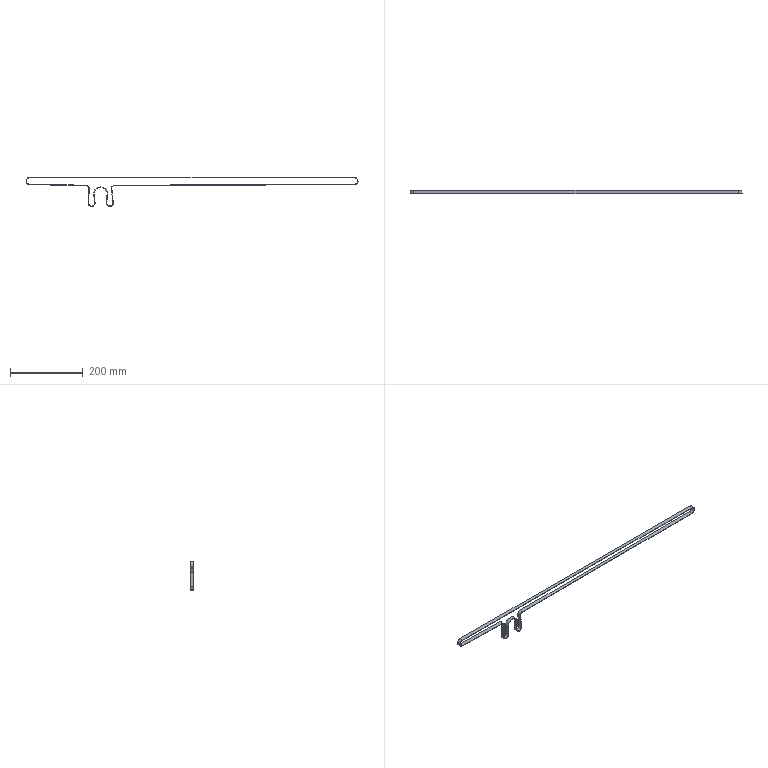Part | STEP file | ROTATION MC_NEW VER-0610_582 | 1 solid | 30 faces | box 910.4 x 10 x 79.4 mm | volume 24385 mm3 | plane 16 | cylinder 14 | commonest cylinder face diameters 17 x6 19.4 x4 14.6 x2 35.6 x1 38 x1
STEP:
#1=CARTESIAN_POINT('',(-271.857,585.703,-62.593));
#2=VERTEX_POINT('',#1);
#3=CARTESIAN_POINT('',(-427.633,585.703,-59.59));
#4=VERTEX_POINT('',#3);
#5=CARTESIAN_POINT('',(-271.857,585.703,-62.593));
#6=DIRECTION('',(-0.9998,0.,0.01928));
#7=VECTOR('',#6,155.805);
#8=LINE('',#5,#7);
#9=EDGE_CURVE('',#2,#4,#8,.T.);
#10=ORIENTED_EDGE('',*,*,#9,.T.);
#11=CARTESIAN_POINT('',(-427.633,575.703,-59.59));
#12=VERTEX_POINT('',#11);
#13=CARTESIAN_POINT('',(-427.633,575.703,-59.59));
#14=DIRECTION('',(0.,1.,0.));
#15=VECTOR('',#14,10.);
#16=LINE('',#13,#15);
#17=EDGE_CURVE('',#12,#4,#16,.T.);
#18=ORIENTED_EDGE('',*,*,#17,.F.);
#19=CARTESIAN_POINT('',(-271.857,575.703,-62.593));
#20=VERTEX_POINT('',#19);
#21=CARTESIAN_POINT('',(-271.857,575.703,-62.593));
#22=DIRECTION('',(-0.9998,0.,0.01928));
#23=VECTOR('',#22,155.805);
#24=LINE('',#21,#23);
#25=EDGE_CURVE('',#20,#12,#24,.T.);
#26=ORIENTED_EDGE('',*,*,#25,.F.);
#27=CARTESIAN_POINT('',(-271.857,575.703,-62.593));
#28=DIRECTION('',(0.,1.,0.));
#29=VECTOR('',#28,10.);
#30=LINE('',#27,#29);
#31=EDGE_CURVE('',#20,#2,#30,.T.);
#32=ORIENTED_EDGE('',*,*,#31,.T.);
#33=EDGE_LOOP('',(#10,#18,#26,#32));
#34=FACE_OUTER_BOUND('',#33,.T.);
#35=CARTESIAN_POINT('',(-271.857,575.703,-62.593));
#36=DIRECTION('',(-0.01928,0.,-0.9998));
#37=DIRECTION('',(-0.9998,0.,0.01928));
#38=AXIS2_PLACEMENT_3D('',#35,#36,#37);
#39=PLANE('',#38);
#40=ADVANCED_FACE('',(#34),#39,.F.);
#41=CARTESIAN_POINT('',(-427.469,585.703,-42.591));
#42=VERTEX_POINT('',#41);
#43=CARTESIAN_POINT('',(-427.469,585.703,-51.091));
#44=DIRECTION('',(0.,1.,0.));
#45=DIRECTION('',(1.,0.,0.));
#46=AXIS2_PLACEMENT_3D('',#43,#44,#45);
#47=CIRCLE('',#46,8.5);
#48=EDGE_CURVE('',#4,#42,#47,.T.);
#49=ORIENTED_EDGE('',*,*,#48,.T.);
#50=CARTESIAN_POINT('',(-427.469,575.703,-42.591));
#51=VERTEX_POINT('',#50);
#52=CARTESIAN_POINT('',(-427.469,575.703,-42.591));
#53=DIRECTION('',(0.,1.,0.));
#54=VECTOR('',#53,10.);
#55=LINE('',#52,#54);
#56=EDGE_CURVE('',#51,#42,#55,.T.);
#57=ORIENTED_EDGE('',*,*,#56,.F.);
#58=CARTESIAN_POINT('',(-427.469,575.703,-51.091));
#59=DIRECTION('',(0.,1.,0.));
#60=DIRECTION('',(1.,0.,0.));
#61=AXIS2_PLACEMENT_3D('',#58,#59,#60);
#62=CIRCLE('',#61,8.5);
#63=EDGE_CURVE('',#12,#51,#62,.T.);
#64=ORIENTED_EDGE('',*,*,#63,.F.);
#65=ORIENTED_EDGE('',*,*,#17,.T.);
#66=EDGE_LOOP('',(#49,#57,#64,#65));
#67=FACE_OUTER_BOUND('',#66,.T.);
#68=CARTESIAN_POINT('',(-427.469,575.703,-51.091));
#69=DIRECTION('',(0.,1.,0.));
#70=DIRECTION('',(0.,0.,1.));
#71=AXIS2_PLACEMENT_3D('',#68,#69,#70);
#72=CYLINDRICAL_SURFACE('',#71,8.5);
#73=ADVANCED_FACE('',(#67),#72,.F.);
#74=CARTESIAN_POINT('',(463.531,585.703,-42.591));
#75=VERTEX_POINT('',#74);
#76=CARTESIAN_POINT('',(-427.469,585.703,-42.591));
#77=DIRECTION('',(1.,0.,0.));
#78=VECTOR('',#77,891.);
#79=LINE('',#76,#78);
#80=EDGE_CURVE('',#42,#75,#79,.T.);
#81=ORIENTED_EDGE('',*,*,#80,.T.);
#82=CARTESIAN_POINT('',(463.531,575.703,-42.591));
#83=VERTEX_POINT('',#82);
#84=CARTESIAN_POINT('',(463.531,575.703,-42.591));
#85=DIRECTION('',(0.,1.,0.));
#86=VECTOR('',#85,10.);
#87=LINE('',#84,#86);
#88=EDGE_CURVE('',#83,#75,#87,.T.);
#89=ORIENTED_EDGE('',*,*,#88,.F.);
#90=CARTESIAN_POINT('',(-427.469,575.703,-42.591));
#91=DIRECTION('',(1.,0.,0.));
#92=VECTOR('',#91,891.);
#93=LINE('',#90,#92);
#94=EDGE_CURVE('',#51,#83,#93,.T.);
#95=ORIENTED_EDGE('',*,*,#94,.F.);
#96=ORIENTED_EDGE('',*,*,#56,.T.);
#97=EDGE_LOOP('',(#81,#89,#95,#96));
#98=FACE_OUTER_BOUND('',#97,.T.);
#99=CARTESIAN_POINT('',(-427.469,575.703,-42.591));
#100=DIRECTION('',(0.,0.,1.));
#101=DIRECTION('',(1.,0.,0.));
#102=AXIS2_PLACEMENT_3D('',#99,#100,#101);
#103=PLANE('',#102);
#104=ADVANCED_FACE('',(#98),#103,.F.);
#105=CARTESIAN_POINT('',(463.569,585.703,-59.591));
#106=VERTEX_POINT('',#105);
#107=CARTESIAN_POINT('',(463.531,585.703,-51.091));
#108=DIRECTION('',(0.,1.,0.));
#109=DIRECTION('',(1.,0.,0.));
#110=AXIS2_PLACEMENT_3D('',#107,#108,#109);
#111=CIRCLE('',#110,8.5);
#112=EDGE_CURVE('',#75,#106,#111,.T.);
#113=ORIENTED_EDGE('',*,*,#112,.T.);
#114=CARTESIAN_POINT('',(463.569,575.703,-59.591));
#115=VERTEX_POINT('',#114);
#116=CARTESIAN_POINT('',(463.569,575.703,-59.591));
#117=DIRECTION('',(0.,1.,0.));
#118=VECTOR('',#117,10.);
#119=LINE('',#116,#118);
#120=EDGE_CURVE('',#115,#106,#119,.T.);
#121=ORIENTED_EDGE('',*,*,#120,.F.);
#122=CARTESIAN_POINT('',(463.531,575.703,-51.091));
#123=DIRECTION('',(0.,1.,0.));
#124=DIRECTION('',(1.,0.,0.));
#125=AXIS2_PLACEMENT_3D('',#122,#123,#124);
#126=CIRCLE('',#125,8.5);
#127=EDGE_CURVE('',#83,#115,#126,.T.);
#128=ORIENTED_EDGE('',*,*,#127,.F.);
#129=ORIENTED_EDGE('',*,*,#88,.T.);
#130=EDGE_LOOP('',(#113,#121,#128,#129));
#131=FACE_OUTER_BOUND('',#130,.T.);
#132=CARTESIAN_POINT('',(463.531,575.703,-51.091));
#133=DIRECTION('',(0.,1.,0.));
#134=DIRECTION('',(0.,0.,1.));
#135=AXIS2_PLACEMENT_3D('',#132,#133,#134);
#136=CYLINDRICAL_SURFACE('',#135,8.5);
#137=ADVANCED_FACE('',(#131),#136,.F.);
#138=CARTESIAN_POINT('',(-194.588,585.703,-62.591));
#139=VERTEX_POINT('',#138);
#140=CARTESIAN_POINT('',(463.569,585.703,-59.591));
#141=DIRECTION('',(-1.,0.,-0.004558));
#142=VECTOR('',#141,658.164);
#143=LINE('',#140,#142);
#144=EDGE_CURVE('',#106,#139,#143,.T.);
#145=ORIENTED_EDGE('',*,*,#144,.T.);
#146=CARTESIAN_POINT('',(-194.588,575.703,-62.591));
#147=VERTEX_POINT('',#146);
#148=CARTESIAN_POINT('',(-194.588,575.703,-62.591));
#149=DIRECTION('',(0.,1.,0.));
#150=VECTOR('',#149,10.);
#151=LINE('',#148,#150);
#152=EDGE_CURVE('',#147,#139,#151,.T.);
#153=ORIENTED_EDGE('',*,*,#152,.F.);
#154=CARTESIAN_POINT('',(463.569,575.703,-59.591));
#155=DIRECTION('',(-1.,0.,-0.004558));
#156=VECTOR('',#155,658.164);
#157=LINE('',#154,#156);
#158=EDGE_CURVE('',#115,#147,#157,.T.);
#159=ORIENTED_EDGE('',*,*,#158,.F.);
#160=ORIENTED_EDGE('',*,*,#120,.T.);
#161=EDGE_LOOP('',(#145,#153,#159,#160));
#162=FACE_OUTER_BOUND('',#161,.T.);
#163=CARTESIAN_POINT('',(463.569,575.703,-59.591));
#164=DIRECTION('',(0.004558,0.,-1.));
#165=DIRECTION('',(-1.,0.,-0.004558));
#166=AXIS2_PLACEMENT_3D('',#163,#164,#165);
#167=PLANE('',#166);
#168=ADVANCED_FACE('',(#162),#167,.F.);
#169=CARTESIAN_POINT('',(-203.001,585.703,-71.989));
#170=VERTEX_POINT('',#169);
#171=CARTESIAN_POINT('',(-194.549,585.703,-71.091));
#172=DIRECTION('',(0.,-1.,0.));
#173=DIRECTION('',(1.,0.,0.));
#174=AXIS2_PLACEMENT_3D('',#171,#172,#173);
#175=CIRCLE('',#174,8.5);
#176=EDGE_CURVE('',#139,#170,#175,.T.);
#177=ORIENTED_EDGE('',*,*,#176,.T.);
#178=CARTESIAN_POINT('',(-203.001,575.703,-71.989));
#179=VERTEX_POINT('',#178);
#180=CARTESIAN_POINT('',(-203.001,575.703,-71.989));
#181=DIRECTION('',(0.,1.,0.));
#182=VECTOR('',#181,10.);
#183=LINE('',#180,#182);
#184=EDGE_CURVE('',#179,#170,#183,.T.);
#185=ORIENTED_EDGE('',*,*,#184,.F.);
#186=CARTESIAN_POINT('',(-194.549,575.703,-71.091));
#187=DIRECTION('',(0.,-1.,0.));
#188=DIRECTION('',(1.,0.,0.));
#189=AXIS2_PLACEMENT_3D('',#186,#187,#188);
#190=CIRCLE('',#189,8.5);
#191=EDGE_CURVE('',#147,#179,#190,.T.);
#192=ORIENTED_EDGE('',*,*,#191,.F.);
#193=ORIENTED_EDGE('',*,*,#152,.T.);
#194=EDGE_LOOP('',(#177,#185,#192,#193));
#195=FACE_OUTER_BOUND('',#194,.T.);
#196=CARTESIAN_POINT('',(-194.549,575.703,-71.091));
#197=DIRECTION('',(0.,1.,0.));
#198=DIRECTION('',(0.,0.,1.));
#199=AXIS2_PLACEMENT_3D('',#196,#197,#198);
#200=CYLINDRICAL_SURFACE('',#199,8.5);
#201=ADVANCED_FACE('',(#195),#200,.T.);
#202=CARTESIAN_POINT('',(-198.942,585.703,-110.193));
#203=VERTEX_POINT('',#202);
#204=CARTESIAN_POINT('',(-203.001,585.703,-71.989));
#205=DIRECTION('',(0.1057,0.,-0.9944));
#206=VECTOR('',#205,38.419);
#207=LINE('',#204,#206);
#208=EDGE_CURVE('',#170,#203,#207,.T.);
#209=ORIENTED_EDGE('',*,*,#208,.T.);
#210=CARTESIAN_POINT('',(-198.942,575.703,-110.193));
#211=VERTEX_POINT('',#210);
#212=CARTESIAN_POINT('',(-198.942,575.703,-110.193));
#213=DIRECTION('',(0.,1.,0.));
#214=VECTOR('',#213,10.);
#215=LINE('',#212,#214);
#216=EDGE_CURVE('',#211,#203,#215,.T.);
#217=ORIENTED_EDGE('',*,*,#216,.F.);
#218=CARTESIAN_POINT('',(-203.001,575.703,-71.989));
#219=DIRECTION('',(0.1057,0.,-0.9944));
#220=VECTOR('',#219,38.419);
#221=LINE('',#218,#220);
#222=EDGE_CURVE('',#179,#211,#221,.T.);
#223=ORIENTED_EDGE('',*,*,#222,.F.);
#224=ORIENTED_EDGE('',*,*,#184,.T.);
#225=EDGE_LOOP('',(#209,#217,#223,#224));
#226=FACE_OUTER_BOUND('',#225,.T.);
#227=CARTESIAN_POINT('',(-203.001,575.703,-71.989));
#228=DIRECTION('',(0.9944,0.,0.1057));
#229=DIRECTION('',(0.1057,0.,-0.9944));
#230=AXIS2_PLACEMENT_3D('',#227,#228,#229);
#231=PLANE('',#230);
#232=ADVANCED_FACE('',(#226),#231,.F.);
#233=CARTESIAN_POINT('',(-215.85,585.703,-110.222));
#234=VERTEX_POINT('',#233);
#235=CARTESIAN_POINT('',(-207.395,585.703,-111.091));
#236=DIRECTION('',(0.,1.,0.));
#237=DIRECTION('',(1.,0.,0.));
#238=AXIS2_PLACEMENT_3D('',#235,#236,#237);
#239=CIRCLE('',#238,8.5);
#240=EDGE_CURVE('',#203,#234,#239,.T.);
#241=ORIENTED_EDGE('',*,*,#240,.T.);
#242=CARTESIAN_POINT('',(-215.85,575.703,-110.222));
#243=VERTEX_POINT('',#242);
#244=CARTESIAN_POINT('',(-215.85,575.703,-110.222));
#245=DIRECTION('',(0.,1.,0.));
#246=VECTOR('',#245,10.);
#247=LINE('',#244,#246);
#248=EDGE_CURVE('',#243,#234,#247,.T.);
#249=ORIENTED_EDGE('',*,*,#248,.F.);
#250=CARTESIAN_POINT('',(-207.395,575.703,-111.091));
#251=DIRECTION('',(0.,1.,0.));
#252=DIRECTION('',(1.,0.,0.));
#253=AXIS2_PLACEMENT_3D('',#250,#251,#252);
#254=CIRCLE('',#253,8.5);
#255=EDGE_CURVE('',#211,#243,#254,.T.);
#256=ORIENTED_EDGE('',*,*,#255,.F.);
#257=ORIENTED_EDGE('',*,*,#216,.T.);
#258=EDGE_LOOP('',(#241,#249,#256,#257));
#259=FACE_OUTER_BOUND('',#258,.T.);
#260=CARTESIAN_POINT('',(-207.395,575.703,-111.091));
#261=DIRECTION('',(0.,1.,0.));
#262=DIRECTION('',(0.001692,0.,-1.));
#263=AXIS2_PLACEMENT_3D('',#260,#261,#262);
#264=CYLINDRICAL_SURFACE('',#263,8.5);
#265=ADVANCED_FACE('',(#259),#264,.F.);
#266=CARTESIAN_POINT('',(-213.569,585.703,-88.035));
#267=VERTEX_POINT('',#266);
#268=CARTESIAN_POINT('',(-215.85,585.703,-110.222));
#269=DIRECTION('',(0.1023,0.,0.9948));
#270=VECTOR('',#269,22.304);
#271=LINE('',#268,#270);
#272=EDGE_CURVE('',#234,#267,#271,.T.);
#273=ORIENTED_EDGE('',*,*,#272,.T.);
#274=CARTESIAN_POINT('',(-213.569,575.703,-88.035));
#275=VERTEX_POINT('',#274);
#276=CARTESIAN_POINT('',(-213.569,575.703,-88.035));
#277=DIRECTION('',(0.,1.,0.));
#278=VECTOR('',#277,10.);
#279=LINE('',#276,#278);
#280=EDGE_CURVE('',#275,#267,#279,.T.);
#281=ORIENTED_EDGE('',*,*,#280,.F.);
#282=CARTESIAN_POINT('',(-215.85,575.703,-110.222));
#283=DIRECTION('',(0.1023,0.,0.9948));
#284=VECTOR('',#283,22.304);
#285=LINE('',#282,#284);
#286=EDGE_CURVE('',#243,#275,#285,.T.);
#287=ORIENTED_EDGE('',*,*,#286,.F.);
#288=ORIENTED_EDGE('',*,*,#248,.T.);
#289=EDGE_LOOP('',(#273,#281,#287,#288));
#290=FACE_OUTER_BOUND('',#289,.T.);
#291=CARTESIAN_POINT('',(-215.85,575.703,-110.222));
#292=DIRECTION('',(-0.9948,0.,0.1023));
#293=DIRECTION('',(0.1023,0.,0.9948));
#294=AXIS2_PLACEMENT_3D('',#291,#292,#293);
#295=PLANE('',#294);
#296=ADVANCED_FACE('',(#290),#295,.F.);
#297=CARTESIAN_POINT('',(-251.356,585.703,-88.16));
#298=VERTEX_POINT('',#297);
#299=CARTESIAN_POINT('',(-232.469,585.703,-86.091));
#300=DIRECTION('',(0.,-1.,0.));
#301=DIRECTION('',(1.,0.,0.));
#302=AXIS2_PLACEMENT_3D('',#299,#300,#301);
#303=CIRCLE('',#302,19.);
#304=EDGE_CURVE('',#267,#298,#303,.T.);
#305=ORIENTED_EDGE('',*,*,#304,.T.);
#306=CARTESIAN_POINT('',(-251.356,575.703,-88.16));
#307=VERTEX_POINT('',#306);
#308=CARTESIAN_POINT('',(-251.356,575.703,-88.16));
#309=DIRECTION('',(0.,1.,0.));
#310=VECTOR('',#309,10.);
#311=LINE('',#308,#310);
#312=EDGE_CURVE('',#307,#298,#311,.T.);
#313=ORIENTED_EDGE('',*,*,#312,.F.);
#314=CARTESIAN_POINT('',(-232.469,575.703,-86.091));
#315=DIRECTION('',(0.,-1.,0.));
#316=DIRECTION('',(1.,0.,0.));
#317=AXIS2_PLACEMENT_3D('',#314,#315,#316);
#318=CIRCLE('',#317,19.);
#319=EDGE_CURVE('',#275,#307,#318,.T.);
#320=ORIENTED_EDGE('',*,*,#319,.F.);
#321=ORIENTED_EDGE('',*,*,#280,.T.);
#322=EDGE_LOOP('',(#305,#313,#320,#321));
#323=FACE_OUTER_BOUND('',#322,.T.);
#324=CARTESIAN_POINT('',(-232.469,575.703,-86.091));
#325=DIRECTION('',(0.,1.,0.));
#326=DIRECTION('',(0.,0.,1.));
#327=AXIS2_PLACEMENT_3D('',#324,#325,#326);
#328=CYLINDRICAL_SURFACE('',#327,19.);
#329=ADVANCED_FACE('',(#323),#328,.T.);
#330=CARTESIAN_POINT('',(-248.945,585.703,-110.166));
#331=VERTEX_POINT('',#330);
#332=CARTESIAN_POINT('',(-251.356,585.703,-88.16));
#333=DIRECTION('',(0.1089,0.,-0.9941));
#334=VECTOR('',#333,22.137);
#335=LINE('',#332,#334);
#336=EDGE_CURVE('',#298,#331,#335,.T.);
#337=ORIENTED_EDGE('',*,*,#336,.T.);
#338=CARTESIAN_POINT('',(-248.945,575.703,-110.166));
#339=VERTEX_POINT('',#338);
#340=CARTESIAN_POINT('',(-248.945,575.703,-110.166));
#341=DIRECTION('',(0.,1.,0.));
#342=VECTOR('',#341,10.);
#343=LINE('',#340,#342);
#344=EDGE_CURVE('',#339,#331,#343,.T.);
#345=ORIENTED_EDGE('',*,*,#344,.F.);
#346=CARTESIAN_POINT('',(-251.356,575.703,-88.16));
#347=DIRECTION('',(0.1089,0.,-0.9941));
#348=VECTOR('',#347,22.137);
#349=LINE('',#346,#348);
#350=EDGE_CURVE('',#307,#339,#349,.T.);
#351=ORIENTED_EDGE('',*,*,#350,.F.);
#352=ORIENTED_EDGE('',*,*,#312,.T.);
#353=EDGE_LOOP('',(#337,#345,#351,#352));
#354=FACE_OUTER_BOUND('',#353,.T.);
#355=CARTESIAN_POINT('',(-251.356,575.703,-88.16));
#356=DIRECTION('',(0.9941,0.,0.1089));
#357=DIRECTION('',(0.1089,0.,-0.9941));
#358=AXIS2_PLACEMENT_3D('',#355,#356,#357);
#359=PLANE('',#358);
#360=ADVANCED_FACE('',(#354),#359,.F.);
#361=CARTESIAN_POINT('',(-265.88,585.703,-110.581));
#362=VERTEX_POINT('',#361);
#363=CARTESIAN_POINT('',(-257.395,585.703,-111.091));
#364=DIRECTION('',(0.,1.,0.));
#365=DIRECTION('',(1.,0.,0.));
#366=AXIS2_PLACEMENT_3D('',#363,#364,#365);
#367=CIRCLE('',#366,8.5);
#368=EDGE_CURVE('',#331,#362,#367,.T.);
#369=ORIENTED_EDGE('',*,*,#368,.T.);
#370=CARTESIAN_POINT('',(-265.88,575.703,-110.581));
#371=VERTEX_POINT('',#370);
#372=CARTESIAN_POINT('',(-265.88,575.703,-110.581));
#373=DIRECTION('',(0.,1.,0.));
#374=VECTOR('',#373,10.);
#375=LINE('',#372,#374);
#376=EDGE_CURVE('',#371,#362,#375,.T.);
#377=ORIENTED_EDGE('',*,*,#376,.F.);
#378=CARTESIAN_POINT('',(-257.395,575.703,-111.091));
#379=DIRECTION('',(0.,1.,0.));
#380=DIRECTION('',(1.,0.,0.));
#381=AXIS2_PLACEMENT_3D('',#378,#379,#380);
#382=CIRCLE('',#381,8.5);
#383=EDGE_CURVE('',#339,#371,#382,.T.);
#384=ORIENTED_EDGE('',*,*,#383,.F.);
#385=ORIENTED_EDGE('',*,*,#344,.T.);
#386=EDGE_LOOP('',(#369,#377,#384,#385));
#387=FACE_OUTER_BOUND('',#386,.T.);
#388=CARTESIAN_POINT('',(-257.395,575.703,-111.091));
#389=DIRECTION('',(0.,1.,0.));
#390=DIRECTION('',(0.02453,0.,-0.9997));
#391=AXIS2_PLACEMENT_3D('',#388,#389,#390);
#392=CYLINDRICAL_SURFACE('',#391,8.5);
#393=ADVANCED_FACE('',(#387),#392,.F.);
#394=CARTESIAN_POINT('',(-263.536,585.703,-71.601));
#395=VERTEX_POINT('',#394);
#396=CARTESIAN_POINT('',(-265.88,585.703,-110.581));
#397=DIRECTION('',(0.06001,0.,0.9982));
#398=VECTOR('',#397,39.05);
#399=LINE('',#396,#398);
#400=EDGE_CURVE('',#362,#395,#399,.T.);
#401=ORIENTED_EDGE('',*,*,#400,.T.);
#402=CARTESIAN_POINT('',(-263.536,575.703,-71.601));
#403=VERTEX_POINT('',#402);
#404=CARTESIAN_POINT('',(-263.536,575.703,-71.601));
#405=DIRECTION('',(0.,1.,0.));
#406=VECTOR('',#405,10.);
#407=LINE('',#404,#406);
#408=EDGE_CURVE('',#403,#395,#407,.T.);
#409=ORIENTED_EDGE('',*,*,#408,.F.);
#410=CARTESIAN_POINT('',(-265.88,575.703,-110.581));
#411=DIRECTION('',(0.06001,0.,0.9982));
#412=VECTOR('',#411,39.05);
#413=LINE('',#410,#412);
#414=EDGE_CURVE('',#371,#403,#413,.T.);
#415=ORIENTED_EDGE('',*,*,#414,.F.);
#416=ORIENTED_EDGE('',*,*,#376,.T.);
#417=EDGE_LOOP('',(#401,#409,#415,#416));
#418=FACE_OUTER_BOUND('',#417,.T.);
#419=CARTESIAN_POINT('',(-265.88,575.703,-110.581));
#420=DIRECTION('',(-0.9982,0.,0.06001));
#421=DIRECTION('',(0.06001,0.,0.9982));
#422=AXIS2_PLACEMENT_3D('',#419,#420,#421);
#423=PLANE('',#422);
#424=ADVANCED_FACE('',(#418),#423,.F.);
#425=CARTESIAN_POINT('',(-272.021,585.703,-71.091));
#426=DIRECTION('',(0.,-1.,0.));
#427=DIRECTION('',(1.,0.,0.));
#428=AXIS2_PLACEMENT_3D('',#425,#426,#427);
#429=CIRCLE('',#428,8.5);
#430=EDGE_CURVE('',#395,#2,#429,.T.);
#431=ORIENTED_EDGE('',*,*,#430,.T.);
#432=ORIENTED_EDGE('',*,*,#31,.F.);
#433=CARTESIAN_POINT('',(-272.021,575.703,-71.091));
#434=DIRECTION('',(0.,-1.,0.));
#435=DIRECTION('',(1.,0.,0.));
#436=AXIS2_PLACEMENT_3D('',#433,#434,#435);
#437=CIRCLE('',#436,8.5);
#438=EDGE_CURVE('',#403,#20,#437,.T.);
#439=ORIENTED_EDGE('',*,*,#438,.F.);
#440=ORIENTED_EDGE('',*,*,#408,.T.);
#441=EDGE_LOOP('',(#431,#432,#439,#440));
#442=FACE_OUTER_BOUND('',#441,.T.);
#443=CARTESIAN_POINT('',(-272.021,575.703,-71.091));
#444=DIRECTION('',(0.,1.,0.));
#445=DIRECTION('',(0.,0.,1.));
#446=AXIS2_PLACEMENT_3D('',#443,#444,#445);
#447=CYLINDRICAL_SURFACE('',#446,8.5);
#448=ADVANCED_FACE('',(#442),#447,.T.);
#449=CARTESIAN_POINT('',(-271.88,585.703,-63.793));
#450=VERTEX_POINT('',#449);
#451=CARTESIAN_POINT('',(-427.656,585.703,-60.789));
#452=VERTEX_POINT('',#451);
#453=CARTESIAN_POINT('',(-271.88,585.703,-63.793));
#454=DIRECTION('',(-0.9998,0.,0.01928));
#455=VECTOR('',#454,155.805);
#456=LINE('',#453,#455);
#457=EDGE_CURVE('',#450,#452,#456,.T.);
#458=ORIENTED_EDGE('',*,*,#457,.F.);
#459=CARTESIAN_POINT('',(-271.88,575.703,-63.793));
#460=VERTEX_POINT('',#459);
#461=CARTESIAN_POINT('',(-271.88,575.703,-63.793));
#462=DIRECTION('',(0.,1.,0.));
#463=VECTOR('',#462,10.);
#464=LINE('',#461,#463);
#465=EDGE_CURVE('',#460,#450,#464,.T.);
#466=ORIENTED_EDGE('',*,*,#465,.F.);
#467=CARTESIAN_POINT('',(-427.656,575.703,-60.789));
#468=VERTEX_POINT('',#467);
#469=CARTESIAN_POINT('',(-271.88,575.703,-63.793));
#470=DIRECTION('',(-0.9998,0.,0.01928));
#471=VECTOR('',#470,155.805);
#472=LINE('',#469,#471);
#473=EDGE_CURVE('',#460,#468,#472,.T.);
#474=ORIENTED_EDGE('',*,*,#473,.T.);
#475=CARTESIAN_POINT('',(-427.656,575.703,-60.789));
#476=DIRECTION('',(0.,1.,0.));
#477=VECTOR('',#476,10.);
#478=LINE('',#475,#477);
#479=EDGE_CURVE('',#468,#452,#478,.T.);
#480=ORIENTED_EDGE('',*,*,#479,.T.);
#481=EDGE_LOOP('',(#458,#466,#474,#480));
#482=FACE_OUTER_BOUND('',#481,.T.);
#483=CARTESIAN_POINT('',(-271.88,575.703,-63.793));
#484=DIRECTION('',(-0.01928,0.,-0.9998));
#485=DIRECTION('',(-0.9998,0.,0.01928));
#486=AXIS2_PLACEMENT_3D('',#483,#484,#485);
#487=PLANE('',#486);
#488=ADVANCED_FACE('',(#482),#487,.T.);
#489=CARTESIAN_POINT('',(-427.469,585.703,-41.391));
#490=VERTEX_POINT('',#489);
#491=CARTESIAN_POINT('',(-427.469,585.703,-51.091));
#492=DIRECTION('',(0.,1.,0.));
#493=DIRECTION('',(0.,0.,1.));
#494=AXIS2_PLACEMENT_3D('',#491,#492,#493);
#495=CIRCLE('',#494,9.7);
#496=EDGE_CURVE('',#452,#490,#495,.T.);
#497=ORIENTED_EDGE('',*,*,#496,.F.);
#498=ORIENTED_EDGE('',*,*,#479,.F.);
#499=CARTESIAN_POINT('',(-427.469,575.703,-41.391));
#500=VERTEX_POINT('',#499);
#501=CARTESIAN_POINT('',(-427.469,575.703,-51.091));
#502=DIRECTION('',(0.,1.,0.));
#503=DIRECTION('',(0.,0.,1.));
#504=AXIS2_PLACEMENT_3D('',#501,#502,#503);
#505=CIRCLE('',#504,9.7);
#506=EDGE_CURVE('',#468,#500,#505,.T.);
#507=ORIENTED_EDGE('',*,*,#506,.T.);
#508=CARTESIAN_POINT('',(-427.469,575.703,-41.391));
#509=DIRECTION('',(0.,1.,0.));
#510=VECTOR('',#509,10.);
#511=LINE('',#508,#510);
#512=EDGE_CURVE('',#500,#490,#511,.T.);
#513=ORIENTED_EDGE('',*,*,#512,.T.);
#514=EDGE_LOOP('',(#497,#498,#507,#513));
#515=FACE_OUTER_BOUND('',#514,.T.);
#516=CARTESIAN_POINT('',(-427.469,575.703,-51.091));
#517=DIRECTION('',(0.,1.,0.));
#518=DIRECTION('',(0.,0.,1.));
#519=AXIS2_PLACEMENT_3D('',#516,#517,#518);
#520=CYLINDRICAL_SURFACE('',#519,9.7);
#521=ADVANCED_FACE('',(#515),#520,.T.);
#522=CARTESIAN_POINT('',(463.531,585.703,-41.391));
#523=VERTEX_POINT('',#522);
#524=CARTESIAN_POINT('',(-427.469,585.703,-41.391));
#525=DIRECTION('',(1.,0.,0.));
#526=VECTOR('',#525,891.);
#527=LINE('',#524,#526);
#528=EDGE_CURVE('',#490,#523,#527,.T.);
#529=ORIENTED_EDGE('',*,*,#528,.F.);
#530=ORIENTED_EDGE('',*,*,#512,.F.);
#531=CARTESIAN_POINT('',(463.531,575.703,-41.391));
#532=VERTEX_POINT('',#531);
#533=CARTESIAN_POINT('',(-427.469,575.703,-41.391));
#534=DIRECTION('',(1.,0.,0.));
#535=VECTOR('',#534,891.);
#536=LINE('',#533,#535);
#537=EDGE_CURVE('',#500,#532,#536,.T.);
#538=ORIENTED_EDGE('',*,*,#537,.T.);
#539=CARTESIAN_POINT('',(463.531,575.703,-41.391));
#540=DIRECTION('',(0.,1.,0.));
#541=VECTOR('',#540,10.);
#542=LINE('',#539,#541);
#543=EDGE_CURVE('',#532,#523,#542,.T.);
#544=ORIENTED_EDGE('',*,*,#543,.T.);
#545=EDGE_LOOP('',(#529,#530,#538,#544));
#546=FACE_OUTER_BOUND('',#545,.T.);
#547=CARTESIAN_POINT('',(-427.469,575.703,-41.391));
#548=DIRECTION('',(0.,0.,1.));
#549=DIRECTION('',(1.,0.,0.));
#550=AXIS2_PLACEMENT_3D('',#547,#548,#549);
#551=PLANE('',#550);
#552=ADVANCED_FACE('',(#546),#551,.T.);
#553=CARTESIAN_POINT('',(463.575,585.703,-60.791));
#554=VERTEX_POINT('',#553);
#555=CARTESIAN_POINT('',(463.531,585.703,-51.091));
#556=DIRECTION('',(0.,1.,0.));
#557=DIRECTION('',(0.,0.,1.));
#558=AXIS2_PLACEMENT_3D('',#555,#556,#557);
#559=CIRCLE('',#558,9.7);
#560=EDGE_CURVE('',#523,#554,#559,.T.);
#561=ORIENTED_EDGE('',*,*,#560,.F.);
#562=ORIENTED_EDGE('',*,*,#543,.F.);
#563=CARTESIAN_POINT('',(463.575,575.703,-60.791));
#564=VERTEX_POINT('',#563);
#565=CARTESIAN_POINT('',(463.531,575.703,-51.091));
#566=DIRECTION('',(0.,1.,0.));
#567=DIRECTION('',(0.,0.,1.));
#568=AXIS2_PLACEMENT_3D('',#565,#566,#567);
#569=CIRCLE('',#568,9.7);
#570=EDGE_CURVE('',#532,#564,#569,.T.);
#571=ORIENTED_EDGE('',*,*,#570,.T.);
#572=CARTESIAN_POINT('',(463.575,575.703,-60.791));
#573=DIRECTION('',(0.,1.,0.));
#574=VECTOR('',#573,10.);
#575=LINE('',#572,#574);
#576=EDGE_CURVE('',#564,#554,#575,.T.);
#577=ORIENTED_EDGE('',*,*,#576,.T.);
#578=EDGE_LOOP('',(#561,#562,#571,#577));
#579=FACE_OUTER_BOUND('',#578,.T.);
#580=CARTESIAN_POINT('',(463.531,575.703,-51.091));
#581=DIRECTION('',(0.,1.,0.));
#582=DIRECTION('',(0.,0.,1.));
#583=AXIS2_PLACEMENT_3D('',#580,#581,#582);
#584=CYLINDRICAL_SURFACE('',#583,9.7);
#585=ADVANCED_FACE('',(#579),#584,.T.);
#586=CARTESIAN_POINT('',(-194.582,585.703,-63.791));
#587=VERTEX_POINT('',#586);
#588=CARTESIAN_POINT('',(463.575,585.703,-60.791));
#589=DIRECTION('',(-1.,0.,-0.004558));
#590=VECTOR('',#589,658.164);
#591=LINE('',#588,#590);
#592=EDGE_CURVE('',#554,#587,#591,.T.);
#593=ORIENTED_EDGE('',*,*,#592,.F.);
#594=ORIENTED_EDGE('',*,*,#576,.F.);
#595=CARTESIAN_POINT('',(-194.582,575.703,-63.791));
#596=VERTEX_POINT('',#595);
#597=CARTESIAN_POINT('',(463.575,575.703,-60.791));
#598=DIRECTION('',(-1.,0.,-0.004558));
#599=VECTOR('',#598,658.164);
#600=LINE('',#597,#599);
#601=EDGE_CURVE('',#564,#596,#600,.T.);
#602=ORIENTED_EDGE('',*,*,#601,.T.);
#603=CARTESIAN_POINT('',(-194.582,575.703,-63.791));
#604=DIRECTION('',(0.,1.,0.));
#605=VECTOR('',#604,10.);
#606=LINE('',#603,#605);
#607=EDGE_CURVE('',#596,#587,#606,.T.);
#608=ORIENTED_EDGE('',*,*,#607,.T.);
#609=EDGE_LOOP('',(#593,#594,#602,#608));
#610=FACE_OUTER_BOUND('',#609,.T.);
#611=CARTESIAN_POINT('',(463.575,575.703,-60.791));
#612=DIRECTION('',(0.004558,0.,-1.));
#613=DIRECTION('',(-1.,0.,-0.004558));
#614=AXIS2_PLACEMENT_3D('',#611,#612,#613);
#615=PLANE('',#614);
#616=ADVANCED_FACE('',(#610),#615,.T.);
#617=CARTESIAN_POINT('',(-201.808,585.703,-71.863));
#618=VERTEX_POINT('',#617);
#619=CARTESIAN_POINT('',(-194.549,585.703,-71.091));
#620=DIRECTION('',(0.,-1.,0.));
#621=DIRECTION('',(0.,0.,1.));
#622=AXIS2_PLACEMENT_3D('',#619,#620,#621);
#623=CIRCLE('',#622,7.3);
#624=EDGE_CURVE('',#587,#618,#623,.T.);
#625=ORIENTED_EDGE('',*,*,#624,.F.);
#626=ORIENTED_EDGE('',*,*,#607,.F.);
#627=CARTESIAN_POINT('',(-201.808,575.703,-71.863));
#628=VERTEX_POINT('',#627);
#629=CARTESIAN_POINT('',(-194.549,575.703,-71.091));
#630=DIRECTION('',(0.,-1.,0.));
#631=DIRECTION('',(0.,0.,1.));
#632=AXIS2_PLACEMENT_3D('',#629,#630,#631);
#633=CIRCLE('',#632,7.3);
#634=EDGE_CURVE('',#596,#628,#633,.T.);
#635=ORIENTED_EDGE('',*,*,#634,.T.);
#636=CARTESIAN_POINT('',(-201.808,575.703,-71.863));
#637=DIRECTION('',(0.,1.,0.));
#638=VECTOR('',#637,10.);
#639=LINE('',#636,#638);
#640=EDGE_CURVE('',#628,#618,#639,.T.);
#641=ORIENTED_EDGE('',*,*,#640,.T.);
#642=EDGE_LOOP('',(#625,#626,#635,#641));
#643=FACE_OUTER_BOUND('',#642,.T.);
#644=CARTESIAN_POINT('',(-194.549,575.703,-71.091));
#645=DIRECTION('',(0.,1.,0.));
#646=DIRECTION('',(0.,0.,1.));
#647=AXIS2_PLACEMENT_3D('',#644,#645,#646);
#648=CYLINDRICAL_SURFACE('',#647,7.3);
#649=ADVANCED_FACE('',(#643),#648,.F.);
#650=CARTESIAN_POINT('',(-197.749,585.703,-110.066));
#651=VERTEX_POINT('',#650);
#652=CARTESIAN_POINT('',(-201.808,585.703,-71.863));
#653=DIRECTION('',(0.1057,0.,-0.9944));
#654=VECTOR('',#653,38.419);
#655=LINE('',#652,#654);
#656=EDGE_CURVE('',#618,#651,#655,.T.);
#657=ORIENTED_EDGE('',*,*,#656,.F.);
#658=ORIENTED_EDGE('',*,*,#640,.F.);
#659=CARTESIAN_POINT('',(-197.749,575.703,-110.066));
#660=VERTEX_POINT('',#659);
#661=CARTESIAN_POINT('',(-201.808,575.703,-71.863));
#662=DIRECTION('',(0.1057,0.,-0.9944));
#663=VECTOR('',#662,38.419);
#664=LINE('',#661,#663);
#665=EDGE_CURVE('',#628,#660,#664,.T.);
#666=ORIENTED_EDGE('',*,*,#665,.T.);
#667=CARTESIAN_POINT('',(-197.749,575.703,-110.066));
#668=DIRECTION('',(0.,1.,0.));
#669=VECTOR('',#668,10.);
#670=LINE('',#667,#669);
#671=EDGE_CURVE('',#660,#651,#670,.T.);
#672=ORIENTED_EDGE('',*,*,#671,.T.);
#673=EDGE_LOOP('',(#657,#658,#666,#672));
#674=FACE_OUTER_BOUND('',#673,.T.);
#675=CARTESIAN_POINT('',(-201.808,575.703,-71.863));
#676=DIRECTION('',(0.9944,0.,0.1057));
#677=DIRECTION('',(0.1057,0.,-0.9944));
#678=AXIS2_PLACEMENT_3D('',#675,#676,#677);
#679=PLANE('',#678);
#680=ADVANCED_FACE('',(#674),#679,.T.);
#681=CARTESIAN_POINT('',(-217.044,585.703,-110.099));
#682=VERTEX_POINT('',#681);
#683=CARTESIAN_POINT('',(-207.395,585.703,-111.091));
#684=DIRECTION('',(0.,1.,0.));
#685=DIRECTION('',(0.,0.,1.));
#686=AXIS2_PLACEMENT_3D('',#683,#684,#685);
#687=CIRCLE('',#686,9.7);
#688=EDGE_CURVE('',#651,#682,#687,.T.);
#689=ORIENTED_EDGE('',*,*,#688,.F.);
#690=ORIENTED_EDGE('',*,*,#671,.F.);
#691=CARTESIAN_POINT('',(-217.044,575.703,-110.099));
#692=VERTEX_POINT('',#691);
#693=CARTESIAN_POINT('',(-207.395,575.703,-111.091));
#694=DIRECTION('',(0.,1.,0.));
#695=DIRECTION('',(0.,0.,1.));
#696=AXIS2_PLACEMENT_3D('',#693,#694,#695);
#697=CIRCLE('',#696,9.7);
#698=EDGE_CURVE('',#660,#692,#697,.T.);
#699=ORIENTED_EDGE('',*,*,#698,.T.);
#700=CARTESIAN_POINT('',(-217.044,575.703,-110.099));
#701=DIRECTION('',(0.,1.,0.));
#702=VECTOR('',#701,10.);
#703=LINE('',#700,#702);
#704=EDGE_CURVE('',#692,#682,#703,.T.);
#705=ORIENTED_EDGE('',*,*,#704,.T.);
#706=EDGE_LOOP('',(#689,#690,#699,#705));
#707=FACE_OUTER_BOUND('',#706,.T.);
#708=CARTESIAN_POINT('',(-207.395,575.703,-111.091));
#709=DIRECTION('',(0.,1.,0.));
#710=DIRECTION('',(0.001692,0.,-1.));
#711=AXIS2_PLACEMENT_3D('',#708,#709,#710);
#712=CYLINDRICAL_SURFACE('',#711,9.7);
#713=ADVANCED_FACE('',(#707),#712,.T.);
#714=CARTESIAN_POINT('',(-214.763,585.703,-87.912));
#715=VERTEX_POINT('',#714);
#716=CARTESIAN_POINT('',(-217.044,585.703,-110.099));
#717=DIRECTION('',(0.1023,0.,0.9948));
#718=VECTOR('',#717,22.304);
#719=LINE('',#716,#718);
#720=EDGE_CURVE('',#682,#715,#719,.T.);
#721=ORIENTED_EDGE('',*,*,#720,.F.);
#722=ORIENTED_EDGE('',*,*,#704,.F.);
#723=CARTESIAN_POINT('',(-214.763,575.703,-87.912));
#724=VERTEX_POINT('',#723);
#725=CARTESIAN_POINT('',(-217.044,575.703,-110.099));
#726=DIRECTION('',(0.1023,0.,0.9948));
#727=VECTOR('',#726,22.304);
#728=LINE('',#725,#727);
#729=EDGE_CURVE('',#692,#724,#728,.T.);
#730=ORIENTED_EDGE('',*,*,#729,.T.);
#731=CARTESIAN_POINT('',(-214.763,575.703,-87.912));
#732=DIRECTION('',(0.,1.,0.));
#733=VECTOR('',#732,10.);
#734=LINE('',#731,#733);
#735=EDGE_CURVE('',#724,#715,#734,.T.);
#736=ORIENTED_EDGE('',*,*,#735,.T.);
#737=EDGE_LOOP('',(#721,#722,#730,#736));
#738=FACE_OUTER_BOUND('',#737,.T.);
#739=CARTESIAN_POINT('',(-217.044,575.703,-110.099));
#740=DIRECTION('',(-0.9948,0.,0.1023));
#741=DIRECTION('',(0.1023,0.,0.9948));
#742=AXIS2_PLACEMENT_3D('',#739,#740,#741);
#743=PLANE('',#742);
#744=ADVANCED_FACE('',(#738),#743,.T.);
#745=CARTESIAN_POINT('',(-250.163,585.703,-88.03));
#746=VERTEX_POINT('',#745);
#747=CARTESIAN_POINT('',(-232.469,585.703,-86.091));
#748=DIRECTION('',(0.,-1.,0.));
#749=DIRECTION('',(0.,0.,1.));
#750=AXIS2_PLACEMENT_3D('',#747,#748,#749);
#751=CIRCLE('',#750,17.8);
#752=EDGE_CURVE('',#715,#746,#751,.T.);
#753=ORIENTED_EDGE('',*,*,#752,.F.);
#754=ORIENTED_EDGE('',*,*,#735,.F.);
#755=CARTESIAN_POINT('',(-250.163,575.703,-88.03));
#756=VERTEX_POINT('',#755);
#757=CARTESIAN_POINT('',(-232.469,575.703,-86.091));
#758=DIRECTION('',(0.,-1.,0.));
#759=DIRECTION('',(0.,0.,1.));
#760=AXIS2_PLACEMENT_3D('',#757,#758,#759);
#761=CIRCLE('',#760,17.8);
#762=EDGE_CURVE('',#724,#756,#761,.T.);
#763=ORIENTED_EDGE('',*,*,#762,.T.);
#764=CARTESIAN_POINT('',(-250.163,575.703,-88.03));
#765=DIRECTION('',(0.,1.,0.));
#766=VECTOR('',#765,10.);
#767=LINE('',#764,#766);
#768=EDGE_CURVE('',#756,#746,#767,.T.);
#769=ORIENTED_EDGE('',*,*,#768,.T.);
#770=EDGE_LOOP('',(#753,#754,#763,#769));
#771=FACE_OUTER_BOUND('',#770,.T.);
#772=CARTESIAN_POINT('',(-232.469,575.703,-86.091));
#773=DIRECTION('',(0.,1.,0.));
#774=DIRECTION('',(0.,0.,1.));
#775=AXIS2_PLACEMENT_3D('',#772,#773,#774);
#776=CYLINDRICAL_SURFACE('',#775,17.8);
#777=ADVANCED_FACE('',(#771),#776,.F.);
#778=CARTESIAN_POINT('',(-247.753,585.703,-110.035));
#779=VERTEX_POINT('',#778);
#780=CARTESIAN_POINT('',(-250.163,585.703,-88.03));
#781=DIRECTION('',(0.1089,0.,-0.9941));
#782=VECTOR('',#781,22.137);
#783=LINE('',#780,#782);
#784=EDGE_CURVE('',#746,#779,#783,.T.);
#785=ORIENTED_EDGE('',*,*,#784,.F.);
#786=ORIENTED_EDGE('',*,*,#768,.F.);
#787=CARTESIAN_POINT('',(-247.753,575.703,-110.035));
#788=VERTEX_POINT('',#787);
#789=CARTESIAN_POINT('',(-250.163,575.703,-88.03));
#790=DIRECTION('',(0.1089,0.,-0.9941));
#791=VECTOR('',#790,22.137);
#792=LINE('',#789,#791);
#793=EDGE_CURVE('',#756,#788,#792,.T.);
#794=ORIENTED_EDGE('',*,*,#793,.T.);
#795=CARTESIAN_POINT('',(-247.753,575.703,-110.035));
#796=DIRECTION('',(0.,1.,0.));
#797=VECTOR('',#796,10.);
#798=LINE('',#795,#797);
#799=EDGE_CURVE('',#788,#779,#798,.T.);
#800=ORIENTED_EDGE('',*,*,#799,.T.);
#801=EDGE_LOOP('',(#785,#786,#794,#800));
#802=FACE_OUTER_BOUND('',#801,.T.);
#803=CARTESIAN_POINT('',(-250.163,575.703,-88.03));
#804=DIRECTION('',(0.9941,0.,0.1089));
#805=DIRECTION('',(0.1089,0.,-0.9941));
#806=AXIS2_PLACEMENT_3D('',#803,#804,#805);
#807=PLANE('',#806);
#808=ADVANCED_FACE('',(#802),#807,.T.);
#809=CARTESIAN_POINT('',(-267.077,585.703,-110.509));
#810=VERTEX_POINT('',#809);
#811=CARTESIAN_POINT('',(-257.395,585.703,-111.091));
#812=DIRECTION('',(0.,1.,0.));
#813=DIRECTION('',(0.,0.,1.));
#814=AXIS2_PLACEMENT_3D('',#811,#812,#813);
#815=CIRCLE('',#814,9.7);
#816=EDGE_CURVE('',#779,#810,#815,.T.);
#817=ORIENTED_EDGE('',*,*,#816,.F.);
#818=ORIENTED_EDGE('',*,*,#799,.F.);
#819=CARTESIAN_POINT('',(-267.077,575.703,-110.509));
#820=VERTEX_POINT('',#819);
#821=CARTESIAN_POINT('',(-257.395,575.703,-111.091));
#822=DIRECTION('',(0.,1.,0.));
#823=DIRECTION('',(0.,0.,1.));
#824=AXIS2_PLACEMENT_3D('',#821,#822,#823);
#825=CIRCLE('',#824,9.7);
#826=EDGE_CURVE('',#788,#820,#825,.T.);
#827=ORIENTED_EDGE('',*,*,#826,.T.);
#828=CARTESIAN_POINT('',(-267.077,575.703,-110.509));
#829=DIRECTION('',(0.,1.,0.));
#830=VECTOR('',#829,10.);
#831=LINE('',#828,#830);
#832=EDGE_CURVE('',#820,#810,#831,.T.);
#833=ORIENTED_EDGE('',*,*,#832,.T.);
#834=EDGE_LOOP('',(#817,#818,#827,#833));
#835=FACE_OUTER_BOUND('',#834,.T.);
#836=CARTESIAN_POINT('',(-257.395,575.703,-111.091));
#837=DIRECTION('',(0.,1.,0.));
#838=DIRECTION('',(0.02453,0.,-0.9997));
#839=AXIS2_PLACEMENT_3D('',#836,#837,#838);
#840=CYLINDRICAL_SURFACE('',#839,9.7);
#841=ADVANCED_FACE('',(#835),#840,.T.);
#842=CARTESIAN_POINT('',(-264.734,585.703,-71.529));
#843=VERTEX_POINT('',#842);
#844=CARTESIAN_POINT('',(-267.077,585.703,-110.509));
#845=DIRECTION('',(0.06001,0.,0.9982));
#846=VECTOR('',#845,39.05);
#847=LINE('',#844,#846);
#848=EDGE_CURVE('',#810,#843,#847,.T.);
#849=ORIENTED_EDGE('',*,*,#848,.F.);
#850=ORIENTED_EDGE('',*,*,#832,.F.);
#851=CARTESIAN_POINT('',(-264.734,575.703,-71.529));
#852=VERTEX_POINT('',#851);
#853=CARTESIAN_POINT('',(-267.077,575.703,-110.509));
#854=DIRECTION('',(0.06001,0.,0.9982));
#855=VECTOR('',#854,39.05);
#856=LINE('',#853,#855);
#857=EDGE_CURVE('',#820,#852,#856,.T.);
#858=ORIENTED_EDGE('',*,*,#857,.T.);
#859=CARTESIAN_POINT('',(-264.734,575.703,-71.529));
#860=DIRECTION('',(0.,1.,0.));
#861=VECTOR('',#860,10.);
#862=LINE('',#859,#861);
#863=EDGE_CURVE('',#852,#843,#862,.T.);
#864=ORIENTED_EDGE('',*,*,#863,.T.);
#865=EDGE_LOOP('',(#849,#850,#858,#864));
#866=FACE_OUTER_BOUND('',#865,.T.);
#867=CARTESIAN_POINT('',(-267.077,575.703,-110.509));
#868=DIRECTION('',(-0.9982,0.,0.06001));
#869=DIRECTION('',(0.06001,0.,0.9982));
#870=AXIS2_PLACEMENT_3D('',#867,#868,#869);
#871=PLANE('',#870);
#872=ADVANCED_FACE('',(#866),#871,.T.);
#873=CARTESIAN_POINT('',(-272.021,585.703,-71.091));
#874=DIRECTION('',(0.,-1.,0.));
#875=DIRECTION('',(0.,0.,1.));
#876=AXIS2_PLACEMENT_3D('',#873,#874,#875);
#877=CIRCLE('',#876,7.3);
#878=EDGE_CURVE('',#843,#450,#877,.T.);
#879=ORIENTED_EDGE('',*,*,#878,.F.);
#880=ORIENTED_EDGE('',*,*,#863,.F.);
#881=CARTESIAN_POINT('',(-272.021,575.703,-71.091));
#882=DIRECTION('',(0.,-1.,0.));
#883=DIRECTION('',(0.,0.,1.));
#884=AXIS2_PLACEMENT_3D('',#881,#882,#883);
#885=CIRCLE('',#884,7.3);
#886=EDGE_CURVE('',#852,#460,#885,.T.);
#887=ORIENTED_EDGE('',*,*,#886,.T.);
#888=ORIENTED_EDGE('',*,*,#465,.T.);
#889=EDGE_LOOP('',(#879,#880,#887,#888));
#890=FACE_OUTER_BOUND('',#889,.T.);
#891=CARTESIAN_POINT('',(-272.021,575.703,-71.091));
#892=DIRECTION('',(0.,1.,0.));
#893=DIRECTION('',(0.,0.,1.));
#894=AXIS2_PLACEMENT_3D('',#891,#892,#893);
#895=CYLINDRICAL_SURFACE('',#894,7.3);
#896=ADVANCED_FACE('',(#890),#895,.F.);
#897=ORIENTED_EDGE('',*,*,#473,.F.);
#898=ORIENTED_EDGE('',*,*,#886,.F.);
#899=ORIENTED_EDGE('',*,*,#857,.F.);
#900=ORIENTED_EDGE('',*,*,#826,.F.);
#901=ORIENTED_EDGE('',*,*,#793,.F.);
#902=ORIENTED_EDGE('',*,*,#762,.F.);
#903=ORIENTED_EDGE('',*,*,#729,.F.);
#904=ORIENTED_EDGE('',*,*,#698,.F.);
#905=ORIENTED_EDGE('',*,*,#665,.F.);
#906=ORIENTED_EDGE('',*,*,#634,.F.);
#907=ORIENTED_EDGE('',*,*,#601,.F.);
#908=ORIENTED_EDGE('',*,*,#570,.F.);
#909=ORIENTED_EDGE('',*,*,#537,.F.);
#910=ORIENTED_EDGE('',*,*,#506,.F.);
#911=EDGE_LOOP('',(#897,#898,#899,#900,#901,#902,#903,#904,#905,#906,#907,#908,#909,#910));
#912=FACE_OUTER_BOUND('',#911,.T.);
#913=ORIENTED_EDGE('',*,*,#25,.T.);
#914=ORIENTED_EDGE('',*,*,#63,.T.);
#915=ORIENTED_EDGE('',*,*,#94,.T.);
#916=ORIENTED_EDGE('',*,*,#127,.T.);
#917=ORIENTED_EDGE('',*,*,#158,.T.);
#918=ORIENTED_EDGE('',*,*,#191,.T.);
#919=ORIENTED_EDGE('',*,*,#222,.T.);
#920=ORIENTED_EDGE('',*,*,#255,.T.);
#921=ORIENTED_EDGE('',*,*,#286,.T.);
#922=ORIENTED_EDGE('',*,*,#319,.T.);
#923=ORIENTED_EDGE('',*,*,#350,.T.);
#924=ORIENTED_EDGE('',*,*,#383,.T.);
#925=ORIENTED_EDGE('',*,*,#414,.T.);
#926=ORIENTED_EDGE('',*,*,#438,.T.);
#927=EDGE_LOOP('',(#913,#914,#915,#916,#917,#918,#919,#920,#921,#922,#923,#924,#925,#926));
#928=FACE_BOUND('',#927,.T.);
#929=CARTESIAN_POINT('',(-271.857,575.703,-62.593));
#930=DIRECTION('',(0.,-1.,0.));
#931=DIRECTION('',(0.,0.,-1.));
#932=AXIS2_PLACEMENT_3D('',#929,#930,#931);
#933=PLANE('',#932);
#934=ADVANCED_FACE('',(#912,#928),#933,.T.);
#935=ORIENTED_EDGE('',*,*,#848,.T.);
#936=ORIENTED_EDGE('',*,*,#878,.T.);
#937=ORIENTED_EDGE('',*,*,#457,.T.);
#938=ORIENTED_EDGE('',*,*,#496,.T.);
#939=ORIENTED_EDGE('',*,*,#528,.T.);
#940=ORIENTED_EDGE('',*,*,#560,.T.);
#941=ORIENTED_EDGE('',*,*,#592,.T.);
#942=ORIENTED_EDGE('',*,*,#624,.T.);
#943=ORIENTED_EDGE('',*,*,#656,.T.);
#944=ORIENTED_EDGE('',*,*,#688,.T.);
#945=ORIENTED_EDGE('',*,*,#720,.T.);
#946=ORIENTED_EDGE('',*,*,#752,.T.);
#947=ORIENTED_EDGE('',*,*,#784,.T.);
#948=ORIENTED_EDGE('',*,*,#816,.T.);
#949=EDGE_LOOP('',(#935,#936,#937,#938,#939,#940,#941,#942,#943,#944,#945,#946,#947,#948));
#950=FACE_OUTER_BOUND('',#949,.T.);
#951=ORIENTED_EDGE('',*,*,#400,.F.);
#952=ORIENTED_EDGE('',*,*,#368,.F.);
#953=ORIENTED_EDGE('',*,*,#336,.F.);
#954=ORIENTED_EDGE('',*,*,#304,.F.);
#955=ORIENTED_EDGE('',*,*,#272,.F.);
#956=ORIENTED_EDGE('',*,*,#240,.F.);
#957=ORIENTED_EDGE('',*,*,#208,.F.);
#958=ORIENTED_EDGE('',*,*,#176,.F.);
#959=ORIENTED_EDGE('',*,*,#144,.F.);
#960=ORIENTED_EDGE('',*,*,#112,.F.);
#961=ORIENTED_EDGE('',*,*,#80,.F.);
#962=ORIENTED_EDGE('',*,*,#48,.F.);
#963=ORIENTED_EDGE('',*,*,#9,.F.);
#964=ORIENTED_EDGE('',*,*,#430,.F.);
#965=EDGE_LOOP('',(#951,#952,#953,#954,#955,#956,#957,#958,#959,#960,#961,#962,#963,#964));
#966=FACE_BOUND('',#965,.T.);
#967=CARTESIAN_POINT('',(-265.88,585.703,-110.581));
#968=DIRECTION('',(0.,-1.,0.));
#969=DIRECTION('',(0.,0.,-1.));
#970=AXIS2_PLACEMENT_3D('',#967,#968,#969);
#971=PLANE('',#970);
#972=ADVANCED_FACE('',(#950,#966),#971,.F.);
#973=CLOSED_SHELL('',(#40,#73,#104,#137,#168,#201,#232,#265,#296,#329,#360,#393,#424,#448,#488,#521,#552,#585,#616,#649,#680,#713,#744,#777,#808,#841,#872,#896,#934,#972));
#974=MANIFOLD_SOLID_BREP('',#973);
#975=(LENGTH_UNIT()NAMED_UNIT(*)SI_UNIT(.MILLI.,.METRE.));
#976=UNCERTAINTY_MEASURE_WITH_UNIT(LENGTH_MEASURE(0.01),#975,'','');
#977=(NAMED_UNIT(*)PLANE_ANGLE_UNIT()SI_UNIT($,.RADIAN.));
#978=(NAMED_UNIT(*)SI_UNIT($,.STERADIAN.)SOLID_ANGLE_UNIT());
#979=(GEOMETRIC_REPRESENTATION_CONTEXT(3)GLOBAL_UNCERTAINTY_ASSIGNED_CONTEXT((#976))GLOBAL_UNIT_ASSIGNED_CONTEXT((#975,#977,#978))REPRESENTATION_CONTEXT('',''));
#980=ADVANCED_BREP_SHAPE_REPRESENTATION('',(#974),#979);